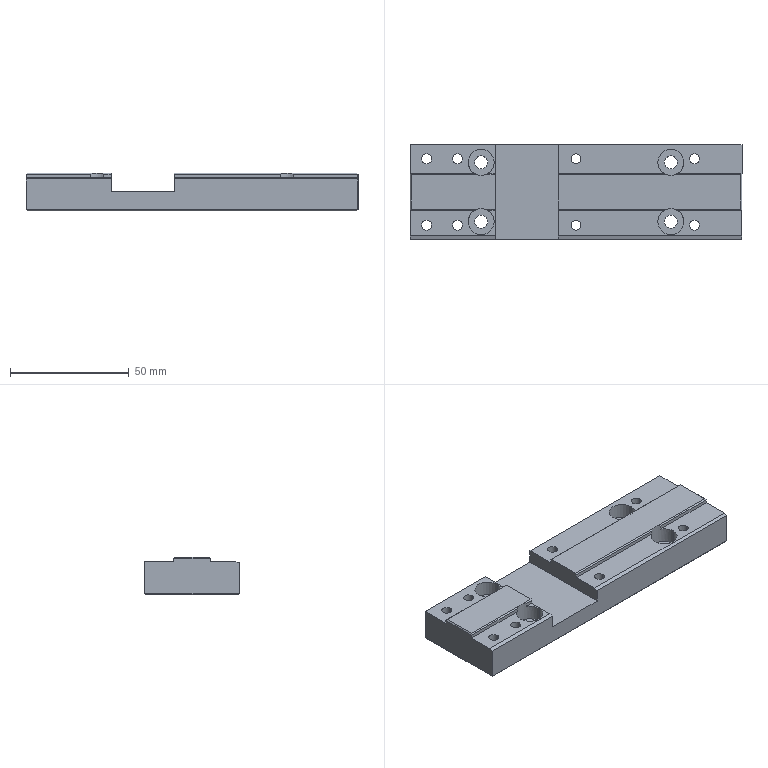Part | STEP file | track (3) | 1 solid | 74 faces | box 140 x 40 x 16 mm | volume 70636 mm3 | plane 42 | cylinder 32 | commonest cylinder face diameters 4.2 x16 5.5 x8 11 x8